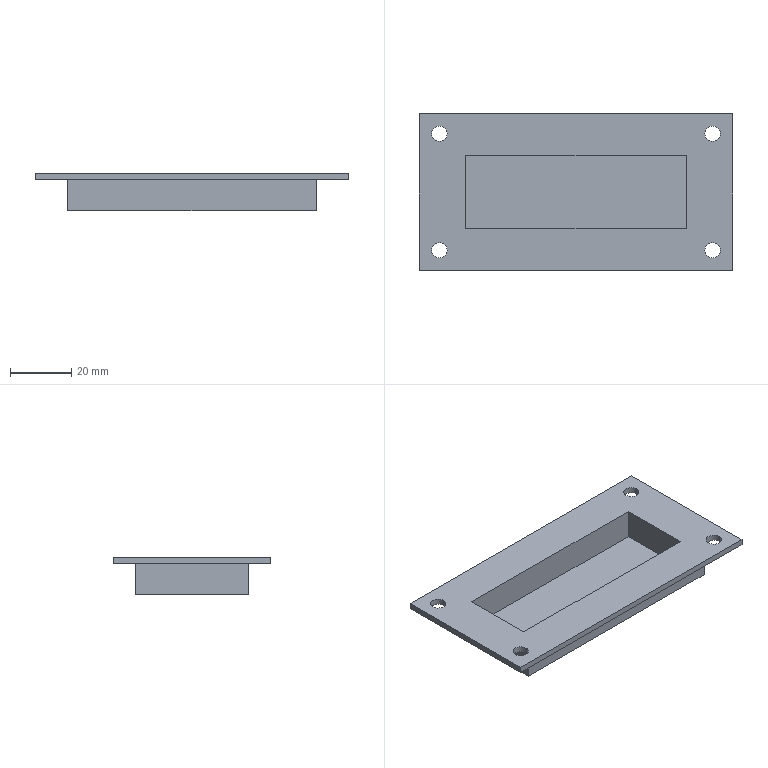Part | STEP file | Hidden handle | 1 solid | 24 faces | box 102 x 51 x 12.2 mm | volume 23536 mm3 | plane 16 | cylinder 8 | commonest cylinder face diameters 5 x8